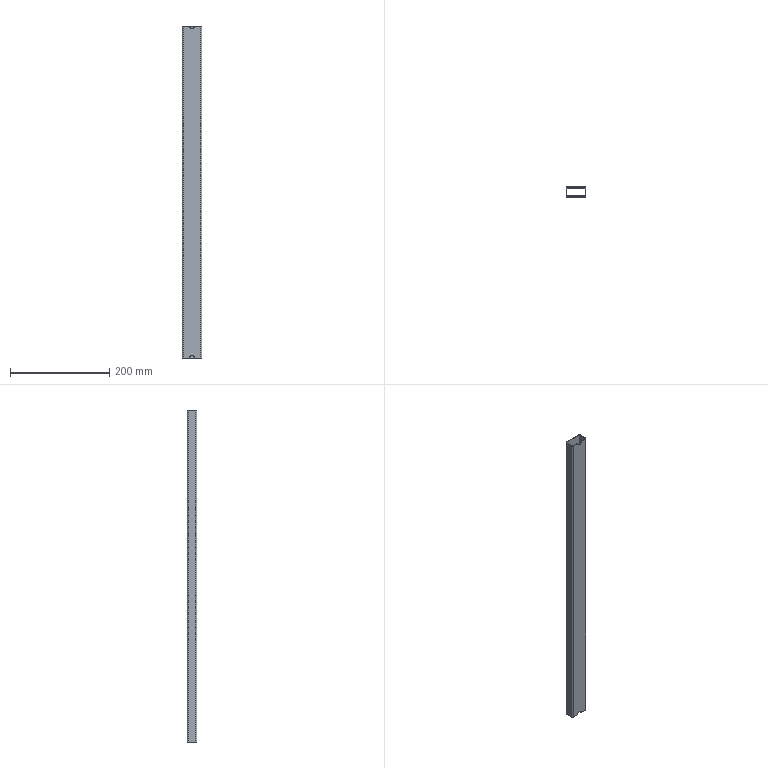Part | STEP file | 7100102 | 1 solid | 20 faces | box 40 x 20 x 670 mm | volume 111433 mm3 | plane 10 | cylinder 10 | commonest cylinder face diameters 2 x4 5 x4 10 x2